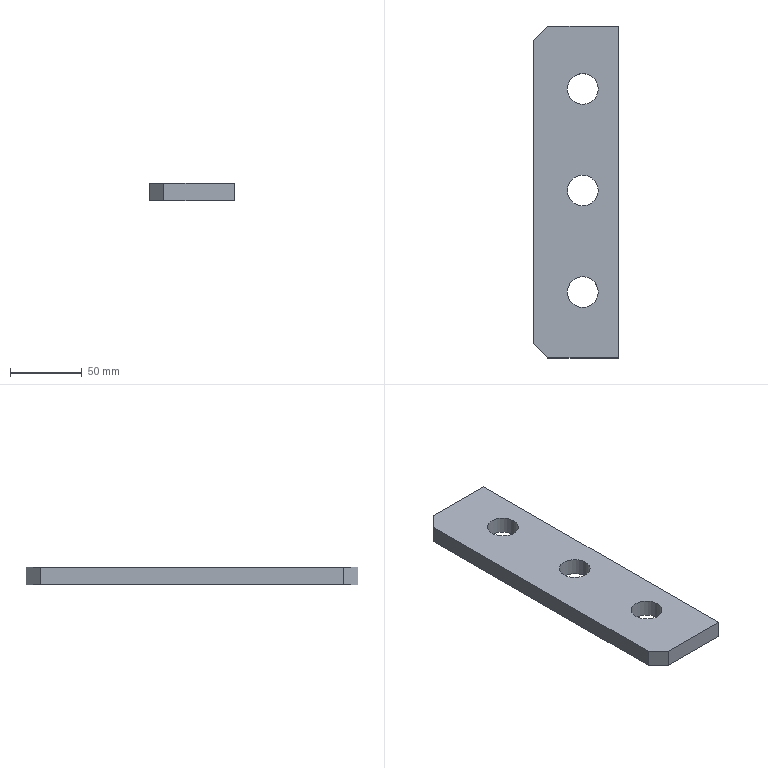Part | STEP file | PN_0032 connecting plate 12t_Default<As Machined> | 1 solid | 11 faces | box 59.5 x 232 x 12 mm | volume 151378 mm3 | plane 8 | cylinder 3 | commonest cylinder face diameters 21.5 x3
STEP:
#1=CARTESIAN_POINT('',(0.,0.,0.));
#2=DIRECTION('',(0.,0.,1.));
#3=DIRECTION('',(1.,0.,0.));
#4=AXIS2_PLACEMENT_3D('',#1,#2,#3);
#5=CARTESIAN_POINT('',(-29.75,-106.,0.));
#6=VERTEX_POINT('',#5);
#7=CARTESIAN_POINT('',(-29.75,-106.,12.));
#8=VERTEX_POINT('',#7);
#9=CARTESIAN_POINT('',(-29.75,-106.,12.));
#10=DIRECTION('',(0.,0.,1.));
#11=VECTOR('',#10,1.);
#12=LINE('',#9,#11);
#13=CARTESIAN_POINT('',(-29.75,-106.,12.));
#14=DIRECTION('',(0.7071,0.7071,0.));
#15=DIRECTION('',(0.,0.,1.));
#16=AXIS2_PLACEMENT_3D('',#13,#14,#15);
#17=PLANE('',#16);
#18=CARTESIAN_POINT('',(0.,0.));
#19=DIRECTION('',(1.,0.));
#20=VECTOR('',#19,1.);
#21=LINE('',#18,#20);
#22=(GEOMETRIC_REPRESENTATION_CONTEXT(2)PARAMETRIC_REPRESENTATION_CONTEXT()REPRESENTATION_CONTEXT('',''));
#23=DEFINITIONAL_REPRESENTATION('',(#21),#22);
#24=PCURVE('',#17,#23);
#25=CARTESIAN_POINT('',(-29.75,116.,12.));
#26=DIRECTION('',(1.,0.,0.));
#27=DIRECTION('',(0.,0.,-1.));
#28=AXIS2_PLACEMENT_3D('',#25,#26,#27);
#29=PLANE('',#28);
#30=CARTESIAN_POINT('',(0.,-222.));
#31=DIRECTION('',(-1.,0.));
#32=VECTOR('',#31,1.);
#33=LINE('',#30,#32);
#34=(GEOMETRIC_REPRESENTATION_CONTEXT(2)PARAMETRIC_REPRESENTATION_CONTEXT()REPRESENTATION_CONTEXT('',''));
#35=DEFINITIONAL_REPRESENTATION('',(#33),#34);
#36=PCURVE('',#29,#35);
#37=SURFACE_CURVE('',#12,(#24,#36),.PCURVE_S1.);
#38=EDGE_CURVE('',#6,#8,#37,.T.);
#39=ORIENTED_EDGE('',*,*,#38,.F.);
#40=CARTESIAN_POINT('',(-19.75,-116.,0.));
#41=VERTEX_POINT('',#40);
#42=CARTESIAN_POINT('',(-29.75,-106.,0.));
#43=DIRECTION('',(-0.7071,0.7071,0.));
#44=VECTOR('',#43,1.);
#45=LINE('',#42,#44);
#46=CARTESIAN_POINT('',(-12.,0.));
#47=DIRECTION('',(0.,-1.));
#48=VECTOR('',#47,1.);
#49=LINE('',#46,#48);
#50=(GEOMETRIC_REPRESENTATION_CONTEXT(2)PARAMETRIC_REPRESENTATION_CONTEXT()REPRESENTATION_CONTEXT('',''));
#51=DEFINITIONAL_REPRESENTATION('',(#49),#50);
#52=PCURVE('',#17,#51);
#53=CARTESIAN_POINT('',(0.,0.,0.));
#54=DIRECTION('',(0.,0.,1.));
#55=DIRECTION('',(1.,0.,0.));
#56=AXIS2_PLACEMENT_3D('',#53,#54,#55);
#57=PLANE('',#56);
#58=CARTESIAN_POINT('',(-29.75,-106.));
#59=DIRECTION('',(-0.7071,0.7071));
#60=VECTOR('',#59,1.);
#61=LINE('',#58,#60);
#62=(GEOMETRIC_REPRESENTATION_CONTEXT(2)PARAMETRIC_REPRESENTATION_CONTEXT()REPRESENTATION_CONTEXT('',''));
#63=DEFINITIONAL_REPRESENTATION('',(#61),#62);
#64=PCURVE('',#57,#63);
#65=SURFACE_CURVE('',#45,(#52,#64),.PCURVE_S1.);
#66=EDGE_CURVE('',#41,#6,#65,.T.);
#67=ORIENTED_EDGE('',*,*,#66,.F.);
#68=CARTESIAN_POINT('',(-19.75,-116.,12.));
#69=VERTEX_POINT('',#68);
#70=CARTESIAN_POINT('',(-19.75,-116.,12.));
#71=DIRECTION('',(0.,0.,-1.));
#72=VECTOR('',#71,1.);
#73=LINE('',#70,#72);
#74=CARTESIAN_POINT('',(0.,14.142));
#75=DIRECTION('',(-1.,0.));
#76=VECTOR('',#75,1.);
#77=LINE('',#74,#76);
#78=(GEOMETRIC_REPRESENTATION_CONTEXT(2)PARAMETRIC_REPRESENTATION_CONTEXT()REPRESENTATION_CONTEXT('',''));
#79=DEFINITIONAL_REPRESENTATION('',(#77),#78);
#80=PCURVE('',#17,#79);
#81=CARTESIAN_POINT('',(-29.75,-116.,12.));
#82=DIRECTION('',(0.,1.,0.));
#83=DIRECTION('',(0.,0.,1.));
#84=AXIS2_PLACEMENT_3D('',#81,#82,#83);
#85=PLANE('',#84);
#86=CARTESIAN_POINT('',(0.,10.));
#87=DIRECTION('',(-1.,0.));
#88=VECTOR('',#87,1.);
#89=LINE('',#86,#88);
#90=(GEOMETRIC_REPRESENTATION_CONTEXT(2)PARAMETRIC_REPRESENTATION_CONTEXT()REPRESENTATION_CONTEXT('',''));
#91=DEFINITIONAL_REPRESENTATION('',(#89),#90);
#92=PCURVE('',#85,#91);
#93=SURFACE_CURVE('',#73,(#80,#92),.PCURVE_S1.);
#94=EDGE_CURVE('',#69,#41,#93,.T.);
#95=ORIENTED_EDGE('',*,*,#94,.F.);
#96=CARTESIAN_POINT('',(-67.875,-67.875,12.));
#97=DIRECTION('',(0.7071,-0.7071,0.));
#98=VECTOR('',#97,1.);
#99=LINE('',#96,#98);
#100=CARTESIAN_POINT('',(0.,-53.917));
#101=DIRECTION('',(0.,1.));
#102=VECTOR('',#101,1.);
#103=LINE('',#100,#102);
#104=(GEOMETRIC_REPRESENTATION_CONTEXT(2)PARAMETRIC_REPRESENTATION_CONTEXT()REPRESENTATION_CONTEXT('',''));
#105=DEFINITIONAL_REPRESENTATION('',(#103),#104);
#106=PCURVE('',#17,#105);
#107=CARTESIAN_POINT('',(0.,0.,12.));
#108=DIRECTION('',(0.,0.,1.));
#109=DIRECTION('',(1.,0.,0.));
#110=AXIS2_PLACEMENT_3D('',#107,#108,#109);
#111=PLANE('',#110);
#112=CARTESIAN_POINT('',(-67.875,-67.875));
#113=DIRECTION('',(0.7071,-0.7071));
#114=VECTOR('',#113,1.);
#115=LINE('',#112,#114);
#116=(GEOMETRIC_REPRESENTATION_CONTEXT(2)PARAMETRIC_REPRESENTATION_CONTEXT()REPRESENTATION_CONTEXT('',''));
#117=DEFINITIONAL_REPRESENTATION('',(#115),#116);
#118=PCURVE('',#111,#117);
#119=SURFACE_CURVE('',#99,(#106,#118),.PCURVE_S1.);
#120=EDGE_CURVE('',#8,#69,#119,.T.);
#121=ORIENTED_EDGE('',*,*,#120,.F.);
#122=EDGE_LOOP('',(#39,#67,#95,#121));
#123=FACE_BOUND('',#122,.T.);
#124=ADVANCED_FACE('',(#123),#17,.F.);
#125=CARTESIAN_POINT('',(-19.75,116.,0.));
#126=VERTEX_POINT('',#125);
#127=CARTESIAN_POINT('',(-19.75,116.,12.));
#128=VERTEX_POINT('',#127);
#129=CARTESIAN_POINT('',(-19.75,116.,12.));
#130=DIRECTION('',(0.,0.,1.));
#131=VECTOR('',#130,1.);
#132=LINE('',#129,#131);
#133=CARTESIAN_POINT('',(-19.75,116.,12.));
#134=DIRECTION('',(0.7071,-0.7071,0.));
#135=DIRECTION('',(0.,0.,1.));
#136=AXIS2_PLACEMENT_3D('',#133,#134,#135);
#137=PLANE('',#136);
#138=CARTESIAN_POINT('',(0.,0.));
#139=DIRECTION('',(1.,0.));
#140=VECTOR('',#139,1.);
#141=LINE('',#138,#140);
#142=(GEOMETRIC_REPRESENTATION_CONTEXT(2)PARAMETRIC_REPRESENTATION_CONTEXT()REPRESENTATION_CONTEXT('',''));
#143=DEFINITIONAL_REPRESENTATION('',(#141),#142);
#144=PCURVE('',#137,#143);
#145=CARTESIAN_POINT('',(-29.75,116.,12.));
#146=DIRECTION('',(0.,-1.,0.));
#147=DIRECTION('',(0.,0.,-1.));
#148=AXIS2_PLACEMENT_3D('',#145,#146,#147);
#149=PLANE('',#148);
#150=CARTESIAN_POINT('',(0.,10.));
#151=DIRECTION('',(-1.,0.));
#152=VECTOR('',#151,1.);
#153=LINE('',#150,#152);
#154=(GEOMETRIC_REPRESENTATION_CONTEXT(2)PARAMETRIC_REPRESENTATION_CONTEXT()REPRESENTATION_CONTEXT('',''));
#155=DEFINITIONAL_REPRESENTATION('',(#153),#154);
#156=PCURVE('',#149,#155);
#157=SURFACE_CURVE('',#132,(#144,#156),.PCURVE_S1.);
#158=EDGE_CURVE('',#126,#128,#157,.T.);
#159=ORIENTED_EDGE('',*,*,#158,.F.);
#160=CARTESIAN_POINT('',(-29.75,106.,0.));
#161=VERTEX_POINT('',#160);
#162=CARTESIAN_POINT('',(-19.75,116.,0.));
#163=DIRECTION('',(0.7071,0.7071,0.));
#164=VECTOR('',#163,1.);
#165=LINE('',#162,#164);
#166=CARTESIAN_POINT('',(-12.,0.));
#167=DIRECTION('',(0.,-1.));
#168=VECTOR('',#167,1.);
#169=LINE('',#166,#168);
#170=(GEOMETRIC_REPRESENTATION_CONTEXT(2)PARAMETRIC_REPRESENTATION_CONTEXT()REPRESENTATION_CONTEXT('',''));
#171=DEFINITIONAL_REPRESENTATION('',(#169),#170);
#172=PCURVE('',#137,#171);
#173=CARTESIAN_POINT('',(-19.75,116.));
#174=DIRECTION('',(0.7071,0.7071));
#175=VECTOR('',#174,1.);
#176=LINE('',#173,#175);
#177=(GEOMETRIC_REPRESENTATION_CONTEXT(2)PARAMETRIC_REPRESENTATION_CONTEXT()REPRESENTATION_CONTEXT('',''));
#178=DEFINITIONAL_REPRESENTATION('',(#176),#177);
#179=PCURVE('',#57,#178);
#180=SURFACE_CURVE('',#165,(#172,#179),.PCURVE_S1.);
#181=EDGE_CURVE('',#161,#126,#180,.T.);
#182=ORIENTED_EDGE('',*,*,#181,.F.);
#183=CARTESIAN_POINT('',(-29.75,106.,12.));
#184=VERTEX_POINT('',#183);
#185=CARTESIAN_POINT('',(-29.75,106.,12.));
#186=DIRECTION('',(0.,0.,-1.));
#187=VECTOR('',#186,1.);
#188=LINE('',#185,#187);
#189=CARTESIAN_POINT('',(0.,14.142));
#190=DIRECTION('',(-1.,0.));
#191=VECTOR('',#190,1.);
#192=LINE('',#189,#191);
#193=(GEOMETRIC_REPRESENTATION_CONTEXT(2)PARAMETRIC_REPRESENTATION_CONTEXT()REPRESENTATION_CONTEXT('',''));
#194=DEFINITIONAL_REPRESENTATION('',(#192),#193);
#195=PCURVE('',#137,#194);
#196=CARTESIAN_POINT('',(0.,-10.));
#197=DIRECTION('',(1.,0.));
#198=VECTOR('',#197,1.);
#199=LINE('',#196,#198);
#200=(GEOMETRIC_REPRESENTATION_CONTEXT(2)PARAMETRIC_REPRESENTATION_CONTEXT()REPRESENTATION_CONTEXT('',''));
#201=DEFINITIONAL_REPRESENTATION('',(#199),#200);
#202=PCURVE('',#29,#201);
#203=SURFACE_CURVE('',#188,(#195,#202),.PCURVE_S1.);
#204=EDGE_CURVE('',#184,#161,#203,.T.);
#205=ORIENTED_EDGE('',*,*,#204,.F.);
#206=CARTESIAN_POINT('',(-67.875,67.875,12.));
#207=DIRECTION('',(-0.7071,-0.7071,0.));
#208=VECTOR('',#207,1.);
#209=LINE('',#206,#208);
#210=CARTESIAN_POINT('',(0.,68.059));
#211=DIRECTION('',(0.,1.));
#212=VECTOR('',#211,1.);
#213=LINE('',#210,#212);
#214=(GEOMETRIC_REPRESENTATION_CONTEXT(2)PARAMETRIC_REPRESENTATION_CONTEXT()REPRESENTATION_CONTEXT('',''));
#215=DEFINITIONAL_REPRESENTATION('',(#213),#214);
#216=PCURVE('',#137,#215);
#217=CARTESIAN_POINT('',(-67.875,67.875));
#218=DIRECTION('',(-0.7071,-0.7071));
#219=VECTOR('',#218,1.);
#220=LINE('',#217,#219);
#221=(GEOMETRIC_REPRESENTATION_CONTEXT(2)PARAMETRIC_REPRESENTATION_CONTEXT()REPRESENTATION_CONTEXT('',''));
#222=DEFINITIONAL_REPRESENTATION('',(#220),#221);
#223=PCURVE('',#111,#222);
#224=SURFACE_CURVE('',#209,(#216,#223),.PCURVE_S1.);
#225=EDGE_CURVE('',#128,#184,#224,.T.);
#226=ORIENTED_EDGE('',*,*,#225,.F.);
#227=EDGE_LOOP('',(#159,#182,#205,#226));
#228=FACE_BOUND('',#227,.T.);
#229=ADVANCED_FACE('',(#228),#137,.F.);
#230=CARTESIAN_POINT('',(29.75,-116.,0.));
#231=VERTEX_POINT('',#230);
#232=CARTESIAN_POINT('',(29.75,116.,0.));
#233=VERTEX_POINT('',#232);
#234=CARTESIAN_POINT('',(29.75,116.,0.));
#235=DIRECTION('',(0.,1.,0.));
#236=VECTOR('',#235,1.);
#237=LINE('',#234,#236);
#238=CARTESIAN_POINT('',(29.75,116.,12.));
#239=DIRECTION('',(-1.,0.,0.));
#240=DIRECTION('',(0.,0.,1.));
#241=AXIS2_PLACEMENT_3D('',#238,#239,#240);
#242=PLANE('',#241);
#243=CARTESIAN_POINT('',(-12.,0.));
#244=DIRECTION('',(0.,1.));
#245=VECTOR('',#244,1.);
#246=LINE('',#243,#245);
#247=(GEOMETRIC_REPRESENTATION_CONTEXT(2)PARAMETRIC_REPRESENTATION_CONTEXT()REPRESENTATION_CONTEXT('',''));
#248=DEFINITIONAL_REPRESENTATION('',(#246),#247);
#249=PCURVE('',#242,#248);
#250=CARTESIAN_POINT('',(29.75,116.));
#251=DIRECTION('',(0.,1.));
#252=VECTOR('',#251,1.);
#253=LINE('',#250,#252);
#254=(GEOMETRIC_REPRESENTATION_CONTEXT(2)PARAMETRIC_REPRESENTATION_CONTEXT()REPRESENTATION_CONTEXT('',''));
#255=DEFINITIONAL_REPRESENTATION('',(#253),#254);
#256=PCURVE('',#57,#255);
#257=SURFACE_CURVE('',#237,(#249,#256),.PCURVE_S1.);
#258=EDGE_CURVE('',#231,#233,#257,.T.);
#259=ORIENTED_EDGE('',*,*,#258,.T.);
#260=CARTESIAN_POINT('',(29.75,116.,12.));
#261=VERTEX_POINT('',#260);
#262=CARTESIAN_POINT('',(29.75,116.,12.));
#263=DIRECTION('',(0.,0.,-1.));
#264=VECTOR('',#263,1.);
#265=LINE('',#262,#264);
#266=CARTESIAN_POINT('',(0.,0.));
#267=DIRECTION('',(-1.,0.));
#268=VECTOR('',#267,1.);
#269=LINE('',#266,#268);
#270=(GEOMETRIC_REPRESENTATION_CONTEXT(2)PARAMETRIC_REPRESENTATION_CONTEXT()REPRESENTATION_CONTEXT('',''));
#271=DEFINITIONAL_REPRESENTATION('',(#269),#270);
#272=PCURVE('',#242,#271);
#273=CARTESIAN_POINT('',(0.,59.5));
#274=DIRECTION('',(1.,0.));
#275=VECTOR('',#274,1.);
#276=LINE('',#273,#275);
#277=(GEOMETRIC_REPRESENTATION_CONTEXT(2)PARAMETRIC_REPRESENTATION_CONTEXT()REPRESENTATION_CONTEXT('',''));
#278=DEFINITIONAL_REPRESENTATION('',(#276),#277);
#279=PCURVE('',#149,#278);
#280=SURFACE_CURVE('',#265,(#272,#279),.PCURVE_S1.);
#281=EDGE_CURVE('',#261,#233,#280,.T.);
#282=ORIENTED_EDGE('',*,*,#281,.F.);
#283=CARTESIAN_POINT('',(29.75,-116.,12.));
#284=VERTEX_POINT('',#283);
#285=CARTESIAN_POINT('',(29.75,116.,12.));
#286=DIRECTION('',(0.,1.,0.));
#287=VECTOR('',#286,1.);
#288=LINE('',#285,#287);
#289=CARTESIAN_POINT('',(0.,0.));
#290=DIRECTION('',(0.,1.));
#291=VECTOR('',#290,1.);
#292=LINE('',#289,#291);
#293=(GEOMETRIC_REPRESENTATION_CONTEXT(2)PARAMETRIC_REPRESENTATION_CONTEXT()REPRESENTATION_CONTEXT('',''));
#294=DEFINITIONAL_REPRESENTATION('',(#292),#293);
#295=PCURVE('',#242,#294);
#296=CARTESIAN_POINT('',(29.75,116.));
#297=DIRECTION('',(0.,1.));
#298=VECTOR('',#297,1.);
#299=LINE('',#296,#298);
#300=(GEOMETRIC_REPRESENTATION_CONTEXT(2)PARAMETRIC_REPRESENTATION_CONTEXT()REPRESENTATION_CONTEXT('',''));
#301=DEFINITIONAL_REPRESENTATION('',(#299),#300);
#302=PCURVE('',#111,#301);
#303=SURFACE_CURVE('',#288,(#295,#302),.PCURVE_S1.);
#304=EDGE_CURVE('',#284,#261,#303,.T.);
#305=ORIENTED_EDGE('',*,*,#304,.F.);
#306=CARTESIAN_POINT('',(29.75,-116.,12.));
#307=DIRECTION('',(0.,0.,-1.));
#308=VECTOR('',#307,1.);
#309=LINE('',#306,#308);
#310=CARTESIAN_POINT('',(0.,-232.));
#311=DIRECTION('',(-1.,0.));
#312=VECTOR('',#311,1.);
#313=LINE('',#310,#312);
#314=(GEOMETRIC_REPRESENTATION_CONTEXT(2)PARAMETRIC_REPRESENTATION_CONTEXT()REPRESENTATION_CONTEXT('',''));
#315=DEFINITIONAL_REPRESENTATION('',(#313),#314);
#316=PCURVE('',#242,#315);
#317=CARTESIAN_POINT('',(0.,59.5));
#318=DIRECTION('',(-1.,0.));
#319=VECTOR('',#318,1.);
#320=LINE('',#317,#319);
#321=(GEOMETRIC_REPRESENTATION_CONTEXT(2)PARAMETRIC_REPRESENTATION_CONTEXT()REPRESENTATION_CONTEXT('',''));
#322=DEFINITIONAL_REPRESENTATION('',(#320),#321);
#323=PCURVE('',#85,#322);
#324=SURFACE_CURVE('',#309,(#316,#323),.PCURVE_S1.);
#325=EDGE_CURVE('',#284,#231,#324,.T.);
#326=ORIENTED_EDGE('',*,*,#325,.T.);
#327=EDGE_LOOP('',(#259,#282,#305,#326));
#328=FACE_BOUND('',#327,.T.);
#329=ADVANCED_FACE('',(#328),#242,.F.);
#330=CARTESIAN_POINT('',(-29.75,116.,0.));
#331=DIRECTION('',(-1.,0.,0.));
#332=VECTOR('',#331,1.);
#333=LINE('',#330,#332);
#334=CARTESIAN_POINT('',(12.,0.));
#335=DIRECTION('',(0.,-1.));
#336=VECTOR('',#335,1.);
#337=LINE('',#334,#336);
#338=(GEOMETRIC_REPRESENTATION_CONTEXT(2)PARAMETRIC_REPRESENTATION_CONTEXT()REPRESENTATION_CONTEXT('',''));
#339=DEFINITIONAL_REPRESENTATION('',(#337),#338);
#340=PCURVE('',#149,#339);
#341=CARTESIAN_POINT('',(-29.75,116.));
#342=DIRECTION('',(-1.,0.));
#343=VECTOR('',#342,1.);
#344=LINE('',#341,#343);
#345=(GEOMETRIC_REPRESENTATION_CONTEXT(2)PARAMETRIC_REPRESENTATION_CONTEXT()REPRESENTATION_CONTEXT('',''));
#346=DEFINITIONAL_REPRESENTATION('',(#344),#345);
#347=PCURVE('',#57,#346);
#348=SURFACE_CURVE('',#333,(#340,#347),.PCURVE_S1.);
#349=EDGE_CURVE('',#233,#126,#348,.T.);
#350=ORIENTED_EDGE('',*,*,#349,.T.);
#351=ORIENTED_EDGE('',*,*,#158,.T.);
#352=CARTESIAN_POINT('',(-29.75,116.,12.));
#353=DIRECTION('',(-1.,0.,0.));
#354=VECTOR('',#353,1.);
#355=LINE('',#352,#354);
#356=CARTESIAN_POINT('',(0.,0.));
#357=DIRECTION('',(0.,-1.));
#358=VECTOR('',#357,1.);
#359=LINE('',#356,#358);
#360=(GEOMETRIC_REPRESENTATION_CONTEXT(2)PARAMETRIC_REPRESENTATION_CONTEXT()REPRESENTATION_CONTEXT('',''));
#361=DEFINITIONAL_REPRESENTATION('',(#359),#360);
#362=PCURVE('',#149,#361);
#363=CARTESIAN_POINT('',(-29.75,116.));
#364=DIRECTION('',(-1.,0.));
#365=VECTOR('',#364,1.);
#366=LINE('',#363,#365);
#367=(GEOMETRIC_REPRESENTATION_CONTEXT(2)PARAMETRIC_REPRESENTATION_CONTEXT()REPRESENTATION_CONTEXT('',''));
#368=DEFINITIONAL_REPRESENTATION('',(#366),#367);
#369=PCURVE('',#111,#368);
#370=SURFACE_CURVE('',#355,(#362,#369),.PCURVE_S1.);
#371=EDGE_CURVE('',#261,#128,#370,.T.);
#372=ORIENTED_EDGE('',*,*,#371,.F.);
#373=ORIENTED_EDGE('',*,*,#281,.T.);
#374=EDGE_LOOP('',(#350,#351,#372,#373));
#375=FACE_BOUND('',#374,.T.);
#376=ADVANCED_FACE('',(#375),#149,.F.);
#377=CARTESIAN_POINT('',(-29.75,116.,0.));
#378=DIRECTION('',(0.,-1.,0.));
#379=VECTOR('',#378,1.);
#380=LINE('',#377,#379);
#381=CARTESIAN_POINT('',(12.,0.));
#382=DIRECTION('',(0.,-1.));
#383=VECTOR('',#382,1.);
#384=LINE('',#381,#383);
#385=(GEOMETRIC_REPRESENTATION_CONTEXT(2)PARAMETRIC_REPRESENTATION_CONTEXT()REPRESENTATION_CONTEXT('',''));
#386=DEFINITIONAL_REPRESENTATION('',(#384),#385);
#387=PCURVE('',#29,#386);
#388=CARTESIAN_POINT('',(-29.75,116.));
#389=DIRECTION('',(0.,-1.));
#390=VECTOR('',#389,1.);
#391=LINE('',#388,#390);
#392=(GEOMETRIC_REPRESENTATION_CONTEXT(2)PARAMETRIC_REPRESENTATION_CONTEXT()REPRESENTATION_CONTEXT('',''));
#393=DEFINITIONAL_REPRESENTATION('',(#391),#392);
#394=PCURVE('',#57,#393);
#395=SURFACE_CURVE('',#380,(#387,#394),.PCURVE_S1.);
#396=EDGE_CURVE('',#161,#6,#395,.T.);
#397=ORIENTED_EDGE('',*,*,#396,.T.);
#398=ORIENTED_EDGE('',*,*,#38,.T.);
#399=CARTESIAN_POINT('',(-29.75,116.,12.));
#400=DIRECTION('',(0.,-1.,0.));
#401=VECTOR('',#400,1.);
#402=LINE('',#399,#401);
#403=CARTESIAN_POINT('',(0.,0.));
#404=DIRECTION('',(0.,-1.));
#405=VECTOR('',#404,1.);
#406=LINE('',#403,#405);
#407=(GEOMETRIC_REPRESENTATION_CONTEXT(2)PARAMETRIC_REPRESENTATION_CONTEXT()REPRESENTATION_CONTEXT('',''));
#408=DEFINITIONAL_REPRESENTATION('',(#406),#407);
#409=PCURVE('',#29,#408);
#410=CARTESIAN_POINT('',(-29.75,116.));
#411=DIRECTION('',(0.,-1.));
#412=VECTOR('',#411,1.);
#413=LINE('',#410,#412);
#414=(GEOMETRIC_REPRESENTATION_CONTEXT(2)PARAMETRIC_REPRESENTATION_CONTEXT()REPRESENTATION_CONTEXT('',''));
#415=DEFINITIONAL_REPRESENTATION('',(#413),#414);
#416=PCURVE('',#111,#415);
#417=SURFACE_CURVE('',#402,(#409,#416),.PCURVE_S1.);
#418=EDGE_CURVE('',#184,#8,#417,.T.);
#419=ORIENTED_EDGE('',*,*,#418,.F.);
#420=ORIENTED_EDGE('',*,*,#204,.T.);
#421=EDGE_LOOP('',(#397,#398,#419,#420));
#422=FACE_BOUND('',#421,.T.);
#423=ADVANCED_FACE('',(#422),#29,.F.);
#424=CARTESIAN_POINT('',(-29.75,-116.,12.));
#425=DIRECTION('',(1.,0.,0.));
#426=VECTOR('',#425,1.);
#427=LINE('',#424,#426);
#428=CARTESIAN_POINT('',(0.,0.));
#429=DIRECTION('',(0.,1.));
#430=VECTOR('',#429,1.);
#431=LINE('',#428,#430);
#432=(GEOMETRIC_REPRESENTATION_CONTEXT(2)PARAMETRIC_REPRESENTATION_CONTEXT()REPRESENTATION_CONTEXT('',''));
#433=DEFINITIONAL_REPRESENTATION('',(#431),#432);
#434=PCURVE('',#85,#433);
#435=CARTESIAN_POINT('',(-29.75,-116.));
#436=DIRECTION('',(1.,0.));
#437=VECTOR('',#436,1.);
#438=LINE('',#435,#437);
#439=(GEOMETRIC_REPRESENTATION_CONTEXT(2)PARAMETRIC_REPRESENTATION_CONTEXT()REPRESENTATION_CONTEXT('',''));
#440=DEFINITIONAL_REPRESENTATION('',(#438),#439);
#441=PCURVE('',#111,#440);
#442=SURFACE_CURVE('',#427,(#434,#441),.PCURVE_S1.);
#443=EDGE_CURVE('',#69,#284,#442,.T.);
#444=ORIENTED_EDGE('',*,*,#443,.F.);
#445=ORIENTED_EDGE('',*,*,#94,.T.);
#446=CARTESIAN_POINT('',(-29.75,-116.,0.));
#447=DIRECTION('',(1.,0.,0.));
#448=VECTOR('',#447,1.);
#449=LINE('',#446,#448);
#450=CARTESIAN_POINT('',(-12.,0.));
#451=DIRECTION('',(0.,1.));
#452=VECTOR('',#451,1.);
#453=LINE('',#450,#452);
#454=(GEOMETRIC_REPRESENTATION_CONTEXT(2)PARAMETRIC_REPRESENTATION_CONTEXT()REPRESENTATION_CONTEXT('',''));
#455=DEFINITIONAL_REPRESENTATION('',(#453),#454);
#456=PCURVE('',#85,#455);
#457=CARTESIAN_POINT('',(-29.75,-116.));
#458=DIRECTION('',(1.,0.));
#459=VECTOR('',#458,1.);
#460=LINE('',#457,#459);
#461=(GEOMETRIC_REPRESENTATION_CONTEXT(2)PARAMETRIC_REPRESENTATION_CONTEXT()REPRESENTATION_CONTEXT('',''));
#462=DEFINITIONAL_REPRESENTATION('',(#460),#461);
#463=PCURVE('',#57,#462);
#464=SURFACE_CURVE('',#449,(#456,#463),.PCURVE_S1.);
#465=EDGE_CURVE('',#41,#231,#464,.T.);
#466=ORIENTED_EDGE('',*,*,#465,.T.);
#467=ORIENTED_EDGE('',*,*,#325,.F.);
#468=EDGE_LOOP('',(#444,#445,#466,#467));
#469=FACE_BOUND('',#468,.T.);
#470=ADVANCED_FACE('',(#469),#85,.F.);
#471=CARTESIAN_POINT('',(15.5,72.,12.));
#472=VERTEX_POINT('',#471);
#473=CARTESIAN_POINT('',(4.75,72.,12.));
#474=DIRECTION('',(0.,0.,1.));
#475=DIRECTION('',(1.,0.,0.));
#476=AXIS2_PLACEMENT_3D('',#473,#474,#475);
#477=CIRCLE('',#476,10.75);
#478=CARTESIAN_POINT('',(4.75,72.));
#479=DIRECTION('',(1.,0.));
#480=AXIS2_PLACEMENT_2D('',#478,#479);
#481=CIRCLE('',#480,10.75);
#482=(GEOMETRIC_REPRESENTATION_CONTEXT(2)PARAMETRIC_REPRESENTATION_CONTEXT()REPRESENTATION_CONTEXT('',''));
#483=DEFINITIONAL_REPRESENTATION('',(#481),#482);
#484=PCURVE('',#111,#483);
#485=CARTESIAN_POINT('',(4.75,72.,12.));
#486=DIRECTION('',(0.,0.,1.));
#487=DIRECTION('',(1.,0.,0.));
#488=AXIS2_PLACEMENT_3D('',#485,#486,#487);
#489=CYLINDRICAL_SURFACE('',#488,10.75);
#490=CARTESIAN_POINT('',(0.,0.));
#491=DIRECTION('',(1.,0.));
#492=VECTOR('',#491,1.);
#493=LINE('',#490,#492);
#494=(GEOMETRIC_REPRESENTATION_CONTEXT(2)PARAMETRIC_REPRESENTATION_CONTEXT()REPRESENTATION_CONTEXT('',''));
#495=DEFINITIONAL_REPRESENTATION('',(#493),#494);
#496=PCURVE('',#489,#495);
#497=SURFACE_CURVE('',#477,(#484,#496),.PCURVE_S1.);
#498=EDGE_CURVE('',#472,#472,#497,.T.);
#499=ORIENTED_EDGE('',*,*,#498,.F.);
#500=EDGE_LOOP('',(#499));
#501=FACE_BOUND('',#500,.T.);
#502=CARTESIAN_POINT('',(15.5,1.,12.));
#503=VERTEX_POINT('',#502);
#504=CARTESIAN_POINT('',(4.75,1.,12.));
#505=DIRECTION('',(0.,0.,1.));
#506=DIRECTION('',(1.,0.,0.));
#507=AXIS2_PLACEMENT_3D('',#504,#505,#506);
#508=CIRCLE('',#507,10.75);
#509=CARTESIAN_POINT('',(4.75,1.));
#510=DIRECTION('',(1.,0.));
#511=AXIS2_PLACEMENT_2D('',#509,#510);
#512=CIRCLE('',#511,10.75);
#513=(GEOMETRIC_REPRESENTATION_CONTEXT(2)PARAMETRIC_REPRESENTATION_CONTEXT()REPRESENTATION_CONTEXT('',''));
#514=DEFINITIONAL_REPRESENTATION('',(#512),#513);
#515=PCURVE('',#111,#514);
#516=CARTESIAN_POINT('',(4.75,1.,12.));
#517=DIRECTION('',(0.,0.,1.));
#518=DIRECTION('',(1.,0.,0.));
#519=AXIS2_PLACEMENT_3D('',#516,#517,#518);
#520=CYLINDRICAL_SURFACE('',#519,10.75);
#521=CARTESIAN_POINT('',(0.,0.));
#522=DIRECTION('',(1.,0.));
#523=VECTOR('',#522,1.);
#524=LINE('',#521,#523);
#525=(GEOMETRIC_REPRESENTATION_CONTEXT(2)PARAMETRIC_REPRESENTATION_CONTEXT()REPRESENTATION_CONTEXT('',''));
#526=DEFINITIONAL_REPRESENTATION('',(#524),#525);
#527=PCURVE('',#520,#526);
#528=SURFACE_CURVE('',#508,(#515,#527),.PCURVE_S1.);
#529=EDGE_CURVE('',#503,#503,#528,.T.);
#530=ORIENTED_EDGE('',*,*,#529,.F.);
#531=EDGE_LOOP('',(#530));
#532=FACE_BOUND('',#531,.T.);
#533=CARTESIAN_POINT('',(15.5,-70.,12.));
#534=VERTEX_POINT('',#533);
#535=CARTESIAN_POINT('',(4.75,-70.,12.));
#536=DIRECTION('',(0.,0.,1.));
#537=DIRECTION('',(1.,0.,0.));
#538=AXIS2_PLACEMENT_3D('',#535,#536,#537);
#539=CIRCLE('',#538,10.75);
#540=CARTESIAN_POINT('',(4.75,-70.));
#541=DIRECTION('',(1.,0.));
#542=AXIS2_PLACEMENT_2D('',#540,#541);
#543=CIRCLE('',#542,10.75);
#544=(GEOMETRIC_REPRESENTATION_CONTEXT(2)PARAMETRIC_REPRESENTATION_CONTEXT()REPRESENTATION_CONTEXT('',''));
#545=DEFINITIONAL_REPRESENTATION('',(#543),#544);
#546=PCURVE('',#111,#545);
#547=CARTESIAN_POINT('',(4.75,-70.,12.));
#548=DIRECTION('',(0.,0.,1.));
#549=DIRECTION('',(1.,0.,0.));
#550=AXIS2_PLACEMENT_3D('',#547,#548,#549);
#551=CYLINDRICAL_SURFACE('',#550,10.75);
#552=CARTESIAN_POINT('',(0.,0.));
#553=DIRECTION('',(1.,0.));
#554=VECTOR('',#553,1.);
#555=LINE('',#552,#554);
#556=(GEOMETRIC_REPRESENTATION_CONTEXT(2)PARAMETRIC_REPRESENTATION_CONTEXT()REPRESENTATION_CONTEXT('',''));
#557=DEFINITIONAL_REPRESENTATION('',(#555),#556);
#558=PCURVE('',#551,#557);
#559=SURFACE_CURVE('',#539,(#546,#558),.PCURVE_S1.);
#560=EDGE_CURVE('',#534,#534,#559,.T.);
#561=ORIENTED_EDGE('',*,*,#560,.F.);
#562=EDGE_LOOP('',(#561));
#563=FACE_BOUND('',#562,.T.);
#564=ORIENTED_EDGE('',*,*,#418,.T.);
#565=ORIENTED_EDGE('',*,*,#120,.T.);
#566=ORIENTED_EDGE('',*,*,#443,.T.);
#567=ORIENTED_EDGE('',*,*,#304,.T.);
#568=ORIENTED_EDGE('',*,*,#371,.T.);
#569=ORIENTED_EDGE('',*,*,#225,.T.);
#570=EDGE_LOOP('',(#564,#565,#566,#567,#568,#569));
#571=FACE_BOUND('',#570,.T.);
#572=ADVANCED_FACE('',(#501,#532,#563,#571),#111,.T.);
#573=CARTESIAN_POINT('',(15.5,72.,0.));
#574=VERTEX_POINT('',#573);
#575=CARTESIAN_POINT('',(4.75,72.,0.));
#576=DIRECTION('',(0.,0.,1.));
#577=DIRECTION('',(1.,0.,0.));
#578=AXIS2_PLACEMENT_3D('',#575,#576,#577);
#579=CIRCLE('',#578,10.75);
#580=CARTESIAN_POINT('',(4.75,72.));
#581=DIRECTION('',(1.,0.));
#582=AXIS2_PLACEMENT_2D('',#580,#581);
#583=CIRCLE('',#582,10.75);
#584=(GEOMETRIC_REPRESENTATION_CONTEXT(2)PARAMETRIC_REPRESENTATION_CONTEXT()REPRESENTATION_CONTEXT('',''));
#585=DEFINITIONAL_REPRESENTATION('',(#583),#584);
#586=PCURVE('',#57,#585);
#587=CARTESIAN_POINT('',(0.,-12.));
#588=DIRECTION('',(1.,0.));
#589=VECTOR('',#588,1.);
#590=LINE('',#587,#589);
#591=(GEOMETRIC_REPRESENTATION_CONTEXT(2)PARAMETRIC_REPRESENTATION_CONTEXT()REPRESENTATION_CONTEXT('',''));
#592=DEFINITIONAL_REPRESENTATION('',(#590),#591);
#593=PCURVE('',#489,#592);
#594=SURFACE_CURVE('',#579,(#586,#593),.PCURVE_S1.);
#595=EDGE_CURVE('',#574,#574,#594,.T.);
#596=ORIENTED_EDGE('',*,*,#595,.T.);
#597=EDGE_LOOP('',(#596));
#598=FACE_BOUND('',#597,.T.);
#599=CARTESIAN_POINT('',(15.5,1.,0.));
#600=VERTEX_POINT('',#599);
#601=CARTESIAN_POINT('',(4.75,1.,0.));
#602=DIRECTION('',(0.,0.,1.));
#603=DIRECTION('',(1.,0.,0.));
#604=AXIS2_PLACEMENT_3D('',#601,#602,#603);
#605=CIRCLE('',#604,10.75);
#606=CARTESIAN_POINT('',(4.75,1.));
#607=DIRECTION('',(1.,0.));
#608=AXIS2_PLACEMENT_2D('',#606,#607);
#609=CIRCLE('',#608,10.75);
#610=(GEOMETRIC_REPRESENTATION_CONTEXT(2)PARAMETRIC_REPRESENTATION_CONTEXT()REPRESENTATION_CONTEXT('',''));
#611=DEFINITIONAL_REPRESENTATION('',(#609),#610);
#612=PCURVE('',#57,#611);
#613=CARTESIAN_POINT('',(0.,-12.));
#614=DIRECTION('',(1.,0.));
#615=VECTOR('',#614,1.);
#616=LINE('',#613,#615);
#617=(GEOMETRIC_REPRESENTATION_CONTEXT(2)PARAMETRIC_REPRESENTATION_CONTEXT()REPRESENTATION_CONTEXT('',''));
#618=DEFINITIONAL_REPRESENTATION('',(#616),#617);
#619=PCURVE('',#520,#618);
#620=SURFACE_CURVE('',#605,(#612,#619),.PCURVE_S1.);
#621=EDGE_CURVE('',#600,#600,#620,.T.);
#622=ORIENTED_EDGE('',*,*,#621,.T.);
#623=EDGE_LOOP('',(#622));
#624=FACE_BOUND('',#623,.T.);
#625=CARTESIAN_POINT('',(15.5,-70.,0.));
#626=VERTEX_POINT('',#625);
#627=CARTESIAN_POINT('',(4.75,-70.,0.));
#628=DIRECTION('',(0.,0.,1.));
#629=DIRECTION('',(1.,0.,0.));
#630=AXIS2_PLACEMENT_3D('',#627,#628,#629);
#631=CIRCLE('',#630,10.75);
#632=CARTESIAN_POINT('',(4.75,-70.));
#633=DIRECTION('',(1.,0.));
#634=AXIS2_PLACEMENT_2D('',#632,#633);
#635=CIRCLE('',#634,10.75);
#636=(GEOMETRIC_REPRESENTATION_CONTEXT(2)PARAMETRIC_REPRESENTATION_CONTEXT()REPRESENTATION_CONTEXT('',''));
#637=DEFINITIONAL_REPRESENTATION('',(#635),#636);
#638=PCURVE('',#57,#637);
#639=CARTESIAN_POINT('',(0.,-12.));
#640=DIRECTION('',(1.,0.));
#641=VECTOR('',#640,1.);
#642=LINE('',#639,#641);
#643=(GEOMETRIC_REPRESENTATION_CONTEXT(2)PARAMETRIC_REPRESENTATION_CONTEXT()REPRESENTATION_CONTEXT('',''));
#644=DEFINITIONAL_REPRESENTATION('',(#642),#643);
#645=PCURVE('',#551,#644);
#646=SURFACE_CURVE('',#631,(#638,#645),.PCURVE_S1.);
#647=EDGE_CURVE('',#626,#626,#646,.T.);
#648=ORIENTED_EDGE('',*,*,#647,.T.);
#649=EDGE_LOOP('',(#648));
#650=FACE_BOUND('',#649,.T.);
#651=ORIENTED_EDGE('',*,*,#465,.F.);
#652=ORIENTED_EDGE('',*,*,#66,.T.);
#653=ORIENTED_EDGE('',*,*,#396,.F.);
#654=ORIENTED_EDGE('',*,*,#181,.T.);
#655=ORIENTED_EDGE('',*,*,#349,.F.);
#656=ORIENTED_EDGE('',*,*,#258,.F.);
#657=EDGE_LOOP('',(#651,#652,#653,#654,#655,#656));
#658=FACE_BOUND('',#657,.T.);
#659=ADVANCED_FACE('',(#598,#624,#650,#658),#57,.F.);
#660=ORIENTED_EDGE('',*,*,#560,.F.);
#661=CARTESIAN_POINT('',(15.5,-70.,0.));
#662=CARTESIAN_POINT('',(15.5,-70.,12.));
#663=B_SPLINE_CURVE_WITH_KNOTS('',1,(#661,#662),.UNSPECIFIED.,.F.,.F.,(2,2),(-12.,0.),.PIECEWISE_BEZIER_KNOTS.);
#664=CARTESIAN_POINT('',(0.,0.));
#665=DIRECTION('',(0.,1.));
#666=VECTOR('',#665,1.);
#667=LINE('',#664,#666);
#668=(GEOMETRIC_REPRESENTATION_CONTEXT(2)PARAMETRIC_REPRESENTATION_CONTEXT()REPRESENTATION_CONTEXT('',''));
#669=DEFINITIONAL_REPRESENTATION('',(#667),#668);
#670=PCURVE('',#551,#669);
#671=CARTESIAN_POINT('',(6.283,0.));
#672=DIRECTION('',(0.,1.));
#673=VECTOR('',#672,1.);
#674=LINE('',#671,#673);
#675=(GEOMETRIC_REPRESENTATION_CONTEXT(2)PARAMETRIC_REPRESENTATION_CONTEXT()REPRESENTATION_CONTEXT('',''));
#676=DEFINITIONAL_REPRESENTATION('',(#674),#675);
#677=PCURVE('',#551,#676);
#678=SEAM_CURVE('',#663,(#670,#677),.PCURVE_S1.);
#679=EDGE_CURVE('',#626,#534,#678,.T.);
#680=ORIENTED_EDGE('',*,*,#679,.F.);
#681=ORIENTED_EDGE('',*,*,#647,.T.);
#682=ORIENTED_EDGE('',*,*,#679,.T.);
#683=EDGE_LOOP('',(#660,#680,#681,#682));
#684=FACE_BOUND('',#683,.F.);
#685=ADVANCED_FACE('',(#684),#551,.F.);
#686=ORIENTED_EDGE('',*,*,#529,.F.);
#687=CARTESIAN_POINT('',(15.5,1.,0.));
#688=CARTESIAN_POINT('',(15.5,1.,12.));
#689=B_SPLINE_CURVE_WITH_KNOTS('',1,(#687,#688),.UNSPECIFIED.,.F.,.F.,(2,2),(-12.,0.),.PIECEWISE_BEZIER_KNOTS.);
#690=CARTESIAN_POINT('',(0.,0.));
#691=DIRECTION('',(0.,1.));
#692=VECTOR('',#691,1.);
#693=LINE('',#690,#692);
#694=(GEOMETRIC_REPRESENTATION_CONTEXT(2)PARAMETRIC_REPRESENTATION_CONTEXT()REPRESENTATION_CONTEXT('',''));
#695=DEFINITIONAL_REPRESENTATION('',(#693),#694);
#696=PCURVE('',#520,#695);
#697=CARTESIAN_POINT('',(6.283,0.));
#698=DIRECTION('',(0.,1.));
#699=VECTOR('',#698,1.);
#700=LINE('',#697,#699);
#701=(GEOMETRIC_REPRESENTATION_CONTEXT(2)PARAMETRIC_REPRESENTATION_CONTEXT()REPRESENTATION_CONTEXT('',''));
#702=DEFINITIONAL_REPRESENTATION('',(#700),#701);
#703=PCURVE('',#520,#702);
#704=SEAM_CURVE('',#689,(#696,#703),.PCURVE_S1.);
#705=EDGE_CURVE('',#600,#503,#704,.T.);
#706=ORIENTED_EDGE('',*,*,#705,.F.);
#707=ORIENTED_EDGE('',*,*,#621,.T.);
#708=ORIENTED_EDGE('',*,*,#705,.T.);
#709=EDGE_LOOP('',(#686,#706,#707,#708));
#710=FACE_BOUND('',#709,.F.);
#711=ADVANCED_FACE('',(#710),#520,.F.);
#712=ORIENTED_EDGE('',*,*,#498,.F.);
#713=CARTESIAN_POINT('',(15.5,72.,0.));
#714=CARTESIAN_POINT('',(15.5,72.,12.));
#715=B_SPLINE_CURVE_WITH_KNOTS('',1,(#713,#714),.UNSPECIFIED.,.F.,.F.,(2,2),(-12.,0.),.PIECEWISE_BEZIER_KNOTS.);
#716=CARTESIAN_POINT('',(0.,0.));
#717=DIRECTION('',(0.,1.));
#718=VECTOR('',#717,1.);
#719=LINE('',#716,#718);
#720=(GEOMETRIC_REPRESENTATION_CONTEXT(2)PARAMETRIC_REPRESENTATION_CONTEXT()REPRESENTATION_CONTEXT('',''));
#721=DEFINITIONAL_REPRESENTATION('',(#719),#720);
#722=PCURVE('',#489,#721);
#723=CARTESIAN_POINT('',(6.283,0.));
#724=DIRECTION('',(0.,1.));
#725=VECTOR('',#724,1.);
#726=LINE('',#723,#725);
#727=(GEOMETRIC_REPRESENTATION_CONTEXT(2)PARAMETRIC_REPRESENTATION_CONTEXT()REPRESENTATION_CONTEXT('',''));
#728=DEFINITIONAL_REPRESENTATION('',(#726),#727);
#729=PCURVE('',#489,#728);
#730=SEAM_CURVE('',#715,(#722,#729),.PCURVE_S1.);
#731=EDGE_CURVE('',#574,#472,#730,.T.);
#732=ORIENTED_EDGE('',*,*,#731,.F.);
#733=ORIENTED_EDGE('',*,*,#595,.T.);
#734=ORIENTED_EDGE('',*,*,#731,.T.);
#735=EDGE_LOOP('',(#712,#732,#733,#734));
#736=FACE_BOUND('',#735,.F.);
#737=ADVANCED_FACE('',(#736),#489,.F.);
#738=CLOSED_SHELL('',(#124,#229,#329,#376,#423,#470,#572,#659,#685,#711,#737));
#739=MANIFOLD_SOLID_BREP('',#738);
#740=(LENGTH_UNIT()NAMED_UNIT(*)SI_UNIT(.MILLI.,.METRE.));
#741=UNCERTAINTY_MEASURE_WITH_UNIT(LENGTH_MEASURE(0.000002),#740,'','');
#742=(NAMED_UNIT(*)PLANE_ANGLE_UNIT()SI_UNIT($,.RADIAN.));
#743=(NAMED_UNIT(*)SI_UNIT($,.STERADIAN.)SOLID_ANGLE_UNIT());
#744=(GEOMETRIC_REPRESENTATION_CONTEXT(3)GLOBAL_UNCERTAINTY_ASSIGNED_CONTEXT((#741))GLOBAL_UNIT_ASSIGNED_CONTEXT((#740,#742,#743))REPRESENTATION_CONTEXT('',''));
#745=ADVANCED_BREP_SHAPE_REPRESENTATION('',(#4,#739),#744);